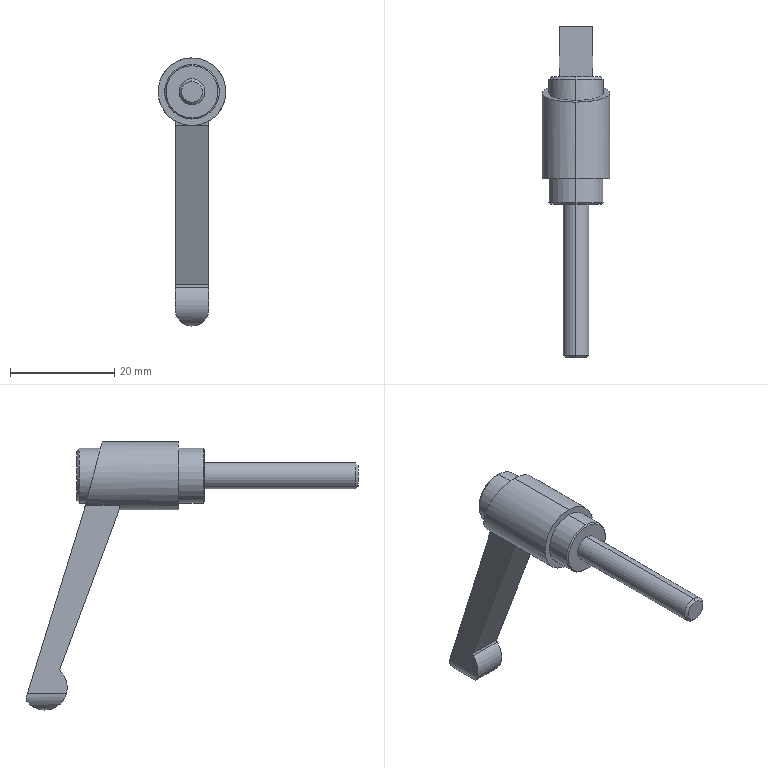Part | NX | features BREP 1 | 1 solid | 31 faces | box 13 x 63.763 x 51.5 mm | volume 4921 mm3 | cylinder 14 | plane 11 | cone 6 | commonest cylinder face diameters 10.5 x4 5 x2 6.5 x2 8.667 x2 13 x2 1 x1
STEP:
#1=CARTESIAN_POINT('',(0.,0.,5.));
#2=VERTEX_POINT('',#1);
#3=CARTESIAN_POINT('',(0.,0.,-5.));
#4=VERTEX_POINT('',#3);
#5=CARTESIAN_POINT('',(0.,0.,0.));
#6=DIRECTION('',(0.,-1.,0.));
#7=DIRECTION('',(0.,0.,1.));
#8=AXIS2_PLACEMENT_3D('',#5,#6,#7);
#9=CIRCLE('',#8,5.);
#10=EDGE_CURVE('',#2,#4,#9,.T.);
#11=ORIENTED_EDGE('',*,*,#10,.T.);
#12=CARTESIAN_POINT('',(0.,0.,0.));
#13=DIRECTION('',(0.,-1.,0.));
#14=DIRECTION('',(0.,0.,-1.));
#15=AXIS2_PLACEMENT_3D('',#12,#13,#14);
#16=CIRCLE('',#15,5.);
#17=EDGE_CURVE('',#4,#2,#16,.T.);
#18=ORIENTED_EDGE('',*,*,#17,.T.);
#19=EDGE_LOOP('',(#11,#18));
#20=FACE_BOUND('',#19,.T.);
#21=CARTESIAN_POINT('',(0.,0.,2.5));
#22=VERTEX_POINT('',#21);
#23=CARTESIAN_POINT('',(0.,0.,-2.5));
#24=VERTEX_POINT('',#23);
#25=CARTESIAN_POINT('',(0.,0.,0.));
#26=DIRECTION('',(0.,1.,0.));
#27=DIRECTION('',(0.,0.,1.));
#28=AXIS2_PLACEMENT_3D('',#25,#26,#27);
#29=CIRCLE('',#28,2.5);
#30=EDGE_CURVE('',#22,#24,#29,.T.);
#31=ORIENTED_EDGE('',*,*,#30,.T.);
#32=CARTESIAN_POINT('',(0.,0.,0.));
#33=DIRECTION('',(0.,1.,0.));
#34=DIRECTION('',(0.,0.,-1.));
#35=AXIS2_PLACEMENT_3D('',#32,#33,#34);
#36=CIRCLE('',#35,2.5);
#37=EDGE_CURVE('',#24,#22,#36,.T.);
#38=ORIENTED_EDGE('',*,*,#37,.T.);
#39=EDGE_LOOP('',(#31,#38));
#40=FACE_BOUND('',#39,.T.);
#41=CARTESIAN_POINT('',(0.,0.,-5.));
#42=DIRECTION('',(0.,1.,0.));
#43=DIRECTION('',(1.,0.,0.));
#44=AXIS2_PLACEMENT_3D('',#41,#42,#43);
#45=PLANE('',#44);
#46=ADVANCED_FACE('',(#20,#40),#45,.F.);
#47=CARTESIAN_POINT('',(0.,0.25,5.25));
#48=VERTEX_POINT('',#47);
#49=CARTESIAN_POINT('',(0.,0.,5.));
#50=DIRECTION('',(0.,0.7071,0.7071));
#51=VECTOR('',#50,1000.);
#52=LINE('',#49,#51);
#53=EDGE_CURVE('',#48,#2,#52,.F.);
#54=ORIENTED_EDGE('',*,*,#53,.T.);
#55=ORIENTED_EDGE('',*,*,#17,.F.);
#56=CARTESIAN_POINT('',(0.,0.25,-5.25));
#57=VERTEX_POINT('',#56);
#58=CARTESIAN_POINT('',(0.,0.,-5.));
#59=DIRECTION('',(0.,0.7071,-0.7071));
#60=VECTOR('',#59,1000.);
#61=LINE('',#58,#60);
#62=EDGE_CURVE('',#57,#4,#61,.F.);
#63=ORIENTED_EDGE('',*,*,#62,.F.);
#64=CARTESIAN_POINT('',(0.,0.25,0.));
#65=DIRECTION('',(0.,-1.,0.));
#66=DIRECTION('',(0.,0.,-1.));
#67=AXIS2_PLACEMENT_3D('',#64,#65,#66);
#68=CIRCLE('',#67,5.25);
#69=EDGE_CURVE('',#57,#48,#68,.T.);
#70=ORIENTED_EDGE('',*,*,#69,.T.);
#71=EDGE_LOOP('',(#54,#55,#63,#70));
#72=FACE_BOUND('',#71,.T.);
#73=CARTESIAN_POINT('',(0.,0.125,0.));
#74=DIRECTION('',(0.,1.,0.));
#75=DIRECTION('',(0.,0.,1.));
#76=AXIS2_PLACEMENT_3D('',#73,#74,#75);
#77=CONICAL_SURFACE('',#76,5.125,0.7854);
#78=ADVANCED_FACE('',(#72),#77,.T.);
#79=CARTESIAN_POINT('',(0.,4.9,5.25));
#80=VERTEX_POINT('',#79);
#81=CARTESIAN_POINT('',(0.,0.25,5.25));
#82=DIRECTION('',(0.,1.,0.));
#83=VECTOR('',#82,1000.);
#84=LINE('',#81,#83);
#85=EDGE_CURVE('',#80,#48,#84,.F.);
#86=ORIENTED_EDGE('',*,*,#85,.T.);
#87=ORIENTED_EDGE('',*,*,#69,.F.);
#88=CARTESIAN_POINT('',(0.,4.9,-5.25));
#89=VERTEX_POINT('',#88);
#90=CARTESIAN_POINT('',(0.,0.25,-5.25));
#91=DIRECTION('',(0.,1.,0.));
#92=VECTOR('',#91,1000.);
#93=LINE('',#90,#92);
#94=EDGE_CURVE('',#89,#57,#93,.F.);
#95=ORIENTED_EDGE('',*,*,#94,.F.);
#96=CARTESIAN_POINT('',(0.,4.9,0.));
#97=DIRECTION('',(0.,1.,0.));
#98=DIRECTION('',(0.,0.,1.));
#99=AXIS2_PLACEMENT_3D('',#96,#97,#98);
#100=CIRCLE('',#99,5.25);
#101=EDGE_CURVE('',#80,#89,#100,.T.);
#102=ORIENTED_EDGE('',*,*,#101,.F.);
#103=EDGE_LOOP('',(#86,#87,#95,#102));
#104=FACE_BOUND('',#103,.T.);
#105=CARTESIAN_POINT('',(0.,-29.5,0.));
#106=DIRECTION('',(0.,1.,0.));
#107=DIRECTION('',(0.,0.,-1.));
#108=AXIS2_PLACEMENT_3D('',#105,#106,#107);
#109=CYLINDRICAL_SURFACE('',#108,5.25);
#110=ADVANCED_FACE('',(#104),#109,.T.);
#111=CARTESIAN_POINT('',(0.,4.9,6.5));
#112=VERTEX_POINT('',#111);
#113=CARTESIAN_POINT('',(0.,4.9,-6.5));
#114=VERTEX_POINT('',#113);
#115=CARTESIAN_POINT('',(0.,4.9,0.));
#116=DIRECTION('',(0.,-1.,0.));
#117=DIRECTION('',(0.,0.,1.));
#118=AXIS2_PLACEMENT_3D('',#115,#116,#117);
#119=CIRCLE('',#118,6.5);
#120=EDGE_CURVE('',#112,#114,#119,.T.);
#121=ORIENTED_EDGE('',*,*,#120,.T.);
#122=CARTESIAN_POINT('',(0.,4.9,0.));
#123=DIRECTION('',(0.,-1.,0.));
#124=DIRECTION('',(0.,0.,-1.));
#125=AXIS2_PLACEMENT_3D('',#122,#123,#124);
#126=CIRCLE('',#125,6.5);
#127=EDGE_CURVE('',#114,#112,#126,.T.);
#128=ORIENTED_EDGE('',*,*,#127,.T.);
#129=EDGE_LOOP('',(#121,#128));
#130=FACE_BOUND('',#129,.T.);
#131=ORIENTED_EDGE('',*,*,#101,.T.);
#132=CARTESIAN_POINT('',(0.,4.9,0.));
#133=DIRECTION('',(0.,1.,0.));
#134=DIRECTION('',(0.,0.,-1.));
#135=AXIS2_PLACEMENT_3D('',#132,#133,#134);
#136=CIRCLE('',#135,5.25);
#137=EDGE_CURVE('',#89,#80,#136,.T.);
#138=ORIENTED_EDGE('',*,*,#137,.T.);
#139=EDGE_LOOP('',(#131,#138));
#140=FACE_BOUND('',#139,.T.);
#141=CARTESIAN_POINT('',(0.,4.9,-6.5));
#142=DIRECTION('',(0.,1.,0.));
#143=DIRECTION('',(1.,0.,0.));
#144=AXIS2_PLACEMENT_3D('',#141,#142,#143);
#145=PLANE('',#144);
#146=ADVANCED_FACE('',(#130,#140),#145,.F.);
#147=CARTESIAN_POINT('',(0.,19.6,6.5));
#148=VERTEX_POINT('',#147);
#149=CARTESIAN_POINT('',(0.,4.9,6.5));
#150=DIRECTION('',(0.,1.,0.));
#151=VECTOR('',#150,1000.);
#152=LINE('',#149,#151);
#153=EDGE_CURVE('',#148,#112,#152,.F.);
#154=ORIENTED_EDGE('',*,*,#153,.T.);
#155=ORIENTED_EDGE('',*,*,#127,.F.);
#156=CARTESIAN_POINT('',(0.,16.333,-6.5));
#157=VERTEX_POINT('',#156);
#158=CARTESIAN_POINT('',(0.,4.9,-6.5));
#159=DIRECTION('',(0.,1.,0.));
#160=VECTOR('',#159,1000.);
#161=LINE('',#158,#160);
#162=EDGE_CURVE('',#157,#114,#161,.F.);
#163=ORIENTED_EDGE('',*,*,#162,.F.);
#164=CARTESIAN_POINT('',(3.25,16.333,-5.629));
#165=VERTEX_POINT('',#164);
#166=CARTESIAN_POINT('',(0.,16.333,0.));
#167=DIRECTION('',(0.,1.,0.));
#168=DIRECTION('',(0.5,0.,-0.866));
#169=AXIS2_PLACEMENT_3D('',#166,#167,#168);
#170=CIRCLE('',#169,6.5);
#171=EDGE_CURVE('',#165,#157,#170,.T.);
#172=ORIENTED_EDGE('',*,*,#171,.F.);
#173=CARTESIAN_POINT('',(3.25,22.814,-5.629));
#174=VERTEX_POINT('',#173);
#175=CARTESIAN_POINT('',(3.25,16.333,-5.629));
#176=DIRECTION('',(0.,1.,0.));
#177=VECTOR('',#176,1000.);
#178=LINE('',#175,#177);
#179=EDGE_CURVE('',#165,#174,#178,.T.);
#180=ORIENTED_EDGE('',*,*,#179,.T.);
#181=CARTESIAN_POINT('',(0.,23.083,-6.5));
#182=VERTEX_POINT('',#181);
#183=CARTESIAN_POINT('',(0.,23.083,-6.5));
#184=CARTESIAN_POINT('',(1.126,23.083,-6.5));
#185=CARTESIAN_POINT('',(2.25,22.992,-6.206));
#186=CARTESIAN_POINT('',(3.25,22.814,-5.629));
#187=B_SPLINE_CURVE_WITH_KNOTS('',3,(#183,#184,#185,#186),.UNSPECIFIED.,.F.,.F.,(4,4),(0.,1.),.UNSPECIFIED.);
#188=EDGE_CURVE('',#174,#182,#187,.F.);
#189=ORIENTED_EDGE('',*,*,#188,.T.);
#190=CARTESIAN_POINT('',(0.,19.6,6.5));
#191=CARTESIAN_POINT('',(0.8361,19.6,6.5));
#192=CARTESIAN_POINT('',(2.441,19.681,6.199));
#193=CARTESIAN_POINT('',(4.728,20.071,4.744));
#194=CARTESIAN_POINT('',(6.224,20.698,2.403));
#195=CARTESIAN_POINT('',(6.638,21.342,0.00000182));
#196=CARTESIAN_POINT('',(6.224,21.986,-2.403));
#197=CARTESIAN_POINT('',(4.728,22.613,-4.744));
#198=CARTESIAN_POINT('',(2.441,23.003,-6.199));
#199=CARTESIAN_POINT('',(0.8365,23.083,-6.5));
#200=CARTESIAN_POINT('',(0.,23.083,-6.5));
#201=B_SPLINE_CURVE_WITH_KNOTS('',3,(#190,#191,#192,#193,#194,#195,#196,#197,#198,#199,#200),.UNSPECIFIED.,.F.,.F.,(4,1,1,1,1,1,1,1,4),(0.,0.125,0.25,0.375,0.5,0.625,0.75,0.875,1.),.UNSPECIFIED.);
#202=EDGE_CURVE('',#182,#148,#201,.F.);
#203=ORIENTED_EDGE('',*,*,#202,.T.);
#204=EDGE_LOOP('',(#154,#155,#163,#172,#180,#189,#203));
#205=FACE_BOUND('',#204,.T.);
#206=CARTESIAN_POINT('',(0.,-29.5,0.));
#207=DIRECTION('',(0.,1.,0.));
#208=DIRECTION('',(0.,0.,-1.));
#209=AXIS2_PLACEMENT_3D('',#206,#207,#208);
#210=CYLINDRICAL_SURFACE('',#209,6.5);
#211=ADVANCED_FACE('',(#205),#210,.T.);
#212=ORIENTED_EDGE('',*,*,#202,.F.);
#213=CARTESIAN_POINT('',(0.,23.083,-6.5));
#214=CARTESIAN_POINT('',(-0.8361,23.083,-6.5));
#215=CARTESIAN_POINT('',(-2.441,23.003,-6.199));
#216=CARTESIAN_POINT('',(-4.728,22.613,-4.744));
#217=CARTESIAN_POINT('',(-6.224,21.986,-2.403));
#218=CARTESIAN_POINT('',(-6.638,21.342,-0.00000182));
#219=CARTESIAN_POINT('',(-6.224,20.698,2.403));
#220=CARTESIAN_POINT('',(-4.728,20.071,4.744));
#221=CARTESIAN_POINT('',(-2.441,19.681,6.199));
#222=CARTESIAN_POINT('',(-0.8365,19.6,6.5));
#223=CARTESIAN_POINT('',(0.,19.6,6.5));
#224=B_SPLINE_CURVE_WITH_KNOTS('',3,(#213,#214,#215,#216,#217,#218,#219,#220,#221,#222,#223),.UNSPECIFIED.,.F.,.F.,(4,1,1,1,1,1,1,1,4),(0.,0.125,0.25,0.375,0.5,0.625,0.75,0.875,1.),.UNSPECIFIED.);
#225=EDGE_CURVE('',#148,#182,#224,.F.);
#226=ORIENTED_EDGE('',*,*,#225,.F.);
#227=EDGE_LOOP('',(#212,#226));
#228=FACE_BOUND('',#227,.T.);
#229=CARTESIAN_POINT('',(0.,19.935,5.25));
#230=VERTEX_POINT('',#229);
#231=CARTESIAN_POINT('',(0.,22.748,-5.25));
#232=VERTEX_POINT('',#231);
#233=CARTESIAN_POINT('',(0.,22.748,-5.25));
#234=CARTESIAN_POINT('',(0.6753,22.748,-5.25));
#235=CARTESIAN_POINT('',(1.972,22.683,-5.007));
#236=CARTESIAN_POINT('',(3.819,22.368,-3.832));
#237=CARTESIAN_POINT('',(5.027,21.862,-1.941));
#238=CARTESIAN_POINT('',(5.361,21.342,-0.00000147));
#239=CARTESIAN_POINT('',(5.027,20.822,1.941));
#240=CARTESIAN_POINT('',(3.819,20.315,3.832));
#241=CARTESIAN_POINT('',(1.972,20.,5.007));
#242=CARTESIAN_POINT('',(0.6757,19.935,5.25));
#243=CARTESIAN_POINT('',(0.,19.935,5.25));
#244=B_SPLINE_CURVE_WITH_KNOTS('',3,(#233,#234,#235,#236,#237,#238,#239,#240,#241,#242,#243),.UNSPECIFIED.,.F.,.F.,(4,1,1,1,1,1,1,1,4),(0.,0.125,0.25,0.375,0.5,0.625,0.75,0.875,1.),.UNSPECIFIED.);
#245=EDGE_CURVE('',#230,#232,#244,.F.);
#246=ORIENTED_EDGE('',*,*,#245,.F.);
#247=CARTESIAN_POINT('',(0.,19.935,5.25));
#248=CARTESIAN_POINT('',(-0.6753,19.935,5.25));
#249=CARTESIAN_POINT('',(-1.972,20.,5.007));
#250=CARTESIAN_POINT('',(-3.819,20.315,3.832));
#251=CARTESIAN_POINT('',(-5.027,20.822,1.941));
#252=CARTESIAN_POINT('',(-5.361,21.342,0.00000147));
#253=CARTESIAN_POINT('',(-5.027,21.862,-1.941));
#254=CARTESIAN_POINT('',(-3.819,22.368,-3.832));
#255=CARTESIAN_POINT('',(-1.972,22.683,-5.007));
#256=CARTESIAN_POINT('',(-0.6757,22.748,-5.25));
#257=CARTESIAN_POINT('',(0.,22.748,-5.25));
#258=B_SPLINE_CURVE_WITH_KNOTS('',3,(#247,#248,#249,#250,#251,#252,#253,#254,#255,#256,#257),.UNSPECIFIED.,.F.,.F.,(4,1,1,1,1,1,1,1,4),(0.,0.125,0.25,0.375,0.5,0.625,0.75,0.875,1.),.UNSPECIFIED.);
#259=EDGE_CURVE('',#232,#230,#258,.F.);
#260=ORIENTED_EDGE('',*,*,#259,.F.);
#261=EDGE_LOOP('',(#246,#260));
#262=FACE_BOUND('',#261,.T.);
#263=CARTESIAN_POINT('',(13.,19.6,6.5));
#264=DIRECTION('',(0.,0.9659,0.2588));
#265=DIRECTION('',(1.,0.,0.));
#266=AXIS2_PLACEMENT_3D('',#263,#264,#265);
#267=PLANE('',#266);
#268=ADVANCED_FACE('',(#228,#262),#267,.T.);
#269=CARTESIAN_POINT('',(-3.25,22.814,-5.629));
#270=VERTEX_POINT('',#269);
#271=CARTESIAN_POINT('',(-3.25,22.814,-5.629));
#272=CARTESIAN_POINT('',(-2.251,22.992,-6.206));
#273=CARTESIAN_POINT('',(-1.127,23.083,-6.5));
#274=CARTESIAN_POINT('',(0.,23.083,-6.5));
#275=B_SPLINE_CURVE_WITH_KNOTS('',3,(#271,#272,#273,#274),.UNSPECIFIED.,.F.,.F.,(4,4),(0.,1.),.UNSPECIFIED.);
#276=EDGE_CURVE('',#182,#270,#275,.F.);
#277=ORIENTED_EDGE('',*,*,#276,.T.);
#278=CARTESIAN_POINT('',(-3.25,16.333,-5.629));
#279=VERTEX_POINT('',#278);
#280=CARTESIAN_POINT('',(-3.25,22.814,-5.629));
#281=DIRECTION('',(0.,-1.,0.));
#282=VECTOR('',#281,1000.);
#283=LINE('',#280,#282);
#284=EDGE_CURVE('',#270,#279,#283,.T.);
#285=ORIENTED_EDGE('',*,*,#284,.T.);
#286=CARTESIAN_POINT('',(0.,16.333,0.));
#287=DIRECTION('',(0.,1.,0.));
#288=DIRECTION('',(0.,0.,-1.));
#289=AXIS2_PLACEMENT_3D('',#286,#287,#288);
#290=CIRCLE('',#289,6.5);
#291=EDGE_CURVE('',#157,#279,#290,.T.);
#292=ORIENTED_EDGE('',*,*,#291,.F.);
#293=ORIENTED_EDGE('',*,*,#162,.T.);
#294=ORIENTED_EDGE('',*,*,#120,.F.);
#295=ORIENTED_EDGE('',*,*,#153,.F.);
#296=ORIENTED_EDGE('',*,*,#225,.T.);
#297=EDGE_LOOP('',(#277,#285,#292,#293,#294,#295,#296));
#298=FACE_BOUND('',#297,.T.);
#299=CARTESIAN_POINT('',(0.,-29.5,0.));
#300=DIRECTION('',(0.,1.,0.));
#301=DIRECTION('',(0.,0.,-1.));
#302=AXIS2_PLACEMENT_3D('',#299,#300,#301);
#303=CYLINDRICAL_SURFACE('',#302,6.5);
#304=ADVANCED_FACE('',(#298),#303,.T.);
#305=ORIENTED_EDGE('',*,*,#291,.T.);
#306=CARTESIAN_POINT('',(-3.25,16.333,-6.5));
#307=VERTEX_POINT('',#306);
#308=CARTESIAN_POINT('',(-3.25,16.333,-6.5));
#309=DIRECTION('',(0.,0.,1.));
#310=VECTOR('',#309,1000.);
#311=LINE('',#308,#310);
#312=EDGE_CURVE('',#307,#279,#311,.T.);
#313=ORIENTED_EDGE('',*,*,#312,.F.);
#314=CARTESIAN_POINT('',(-3.25,16.333,-6.5));
#315=DIRECTION('',(1.,0.,0.));
#316=VECTOR('',#315,1000.);
#317=LINE('',#314,#316);
#318=EDGE_CURVE('',#307,#157,#317,.T.);
#319=ORIENTED_EDGE('',*,*,#318,.T.);
#320=EDGE_LOOP('',(#305,#313,#319));
#321=FACE_BOUND('',#320,.T.);
#322=CARTESIAN_POINT('',(3.25,16.333,0.));
#323=DIRECTION('',(0.,1.,0.));
#324=DIRECTION('',(1.,0.,0.));
#325=AXIS2_PLACEMENT_3D('',#322,#323,#324);
#326=PLANE('',#325);
#327=ADVANCED_FACE('',(#321),#326,.F.);
#328=CARTESIAN_POINT('',(3.25,27.716,-37.076));
#329=VERTEX_POINT('',#328);
#330=CARTESIAN_POINT('',(-3.25,27.716,-37.076));
#331=VERTEX_POINT('',#330);
#332=CARTESIAN_POINT('',(3.25,27.716,-37.076));
#333=DIRECTION('',(-1.,0.,0.));
#334=VECTOR('',#333,1000.);
#335=LINE('',#332,#334);
#336=EDGE_CURVE('',#329,#331,#335,.T.);
#337=ORIENTED_EDGE('',*,*,#336,.F.);
#338=CARTESIAN_POINT('',(3.25,16.333,-6.5));
#339=VERTEX_POINT('',#338);
#340=CARTESIAN_POINT('',(3.25,16.333,-6.5));
#341=DIRECTION('',(0.,0.3489,-0.9372));
#342=VECTOR('',#341,1000.);
#343=LINE('',#340,#342);
#344=EDGE_CURVE('',#339,#329,#343,.T.);
#345=ORIENTED_EDGE('',*,*,#344,.F.);
#346=CARTESIAN_POINT('',(0.,16.333,-6.5));
#347=DIRECTION('',(1.,0.,0.));
#348=VECTOR('',#347,1000.);
#349=LINE('',#346,#348);
#350=EDGE_CURVE('',#157,#339,#349,.T.);
#351=ORIENTED_EDGE('',*,*,#350,.F.);
#352=ORIENTED_EDGE('',*,*,#318,.F.);
#353=CARTESIAN_POINT('',(-3.25,27.716,-37.076));
#354=DIRECTION('',(0.,-0.3489,0.9372));
#355=VECTOR('',#354,1000.);
#356=LINE('',#353,#355);
#357=EDGE_CURVE('',#331,#307,#356,.T.);
#358=ORIENTED_EDGE('',*,*,#357,.F.);
#359=EDGE_LOOP('',(#337,#345,#351,#352,#358));
#360=FACE_BOUND('',#359,.T.);
#361=CARTESIAN_POINT('',(3.25,16.333,-6.5));
#362=DIRECTION('',(0.,0.9372,0.3489));
#363=DIRECTION('',(1.,0.,0.));
#364=AXIS2_PLACEMENT_3D('',#361,#362,#363);
#365=PLANE('',#364);
#366=ADVANCED_FACE('',(#360),#365,.F.);
#367=CARTESIAN_POINT('',(-3.25,26.471,-41.75));
#368=VERTEX_POINT('',#367);
#369=CARTESIAN_POINT('',(-3.25,27.602,-37.604));
#370=VERTEX_POINT('',#369);
#371=CARTESIAN_POINT('',(-3.25,30.667,-40.667));
#372=DIRECTION('',(-1.,0.,0.));
#373=DIRECTION('',(0.,-0.9682,-0.25));
#374=AXIS2_PLACEMENT_3D('',#371,#372,#373);
#375=CIRCLE('',#374,4.333);
#376=EDGE_CURVE('',#368,#370,#375,.T.);
#377=ORIENTED_EDGE('',*,*,#376,.T.);
#378=CARTESIAN_POINT('',(-3.25,27.248,-37.25));
#379=DIRECTION('',(1.,0.,0.));
#380=DIRECTION('',(0.,0.7073,-0.7069));
#381=AXIS2_PLACEMENT_3D('',#378,#379,#380);
#382=CIRCLE('',#381,0.5);
#383=EDGE_CURVE('',#370,#331,#382,.T.);
#384=ORIENTED_EDGE('',*,*,#383,.T.);
#385=ORIENTED_EDGE('',*,*,#357,.T.);
#386=ORIENTED_EDGE('',*,*,#312,.T.);
#387=ORIENTED_EDGE('',*,*,#284,.F.);
#388=CARTESIAN_POINT('',(-3.25,33.994,-41.75));
#389=VERTEX_POINT('',#388);
#390=CARTESIAN_POINT('',(-3.25,22.814,-5.629));
#391=DIRECTION('',(0.,0.2957,-0.9553));
#392=VECTOR('',#391,1000.);
#393=LINE('',#390,#392);
#394=EDGE_CURVE('',#270,#389,#393,.T.);
#395=ORIENTED_EDGE('',*,*,#394,.T.);
#396=CARTESIAN_POINT('',(-3.25,26.471,-41.75));
#397=DIRECTION('',(0.,1.,0.));
#398=VECTOR('',#397,1000.);
#399=LINE('',#396,#398);
#400=EDGE_CURVE('',#368,#389,#399,.T.);
#401=ORIENTED_EDGE('',*,*,#400,.F.);
#402=EDGE_LOOP('',(#377,#384,#385,#386,#387,#395,#401));
#403=FACE_BOUND('',#402,.T.);
#404=CARTESIAN_POINT('',(-3.25,27.248,-37.25));
#405=DIRECTION('',(1.,0.,0.));
#406=DIRECTION('',(0.,1.,0.));
#407=AXIS2_PLACEMENT_3D('',#404,#405,#406);
#408=PLANE('',#407);
#409=ADVANCED_FACE('',(#403),#408,.F.);
#410=CARTESIAN_POINT('',(-2.806,34.038,-43.389));
#411=VERTEX_POINT('',#410);
#412=CARTESIAN_POINT('',(0.,30.667,-45.));
#413=VERTEX_POINT('',#412);
#414=CARTESIAN_POINT('',(-2.806,34.038,-43.389));
#415=CARTESIAN_POINT('',(-2.678,33.861,-43.609));
#416=CARTESIAN_POINT('',(-2.372,33.462,-44.023));
#417=CARTESIAN_POINT('',(-1.814,32.783,-44.467));
#418=CARTESIAN_POINT('',(-1.358,32.243,-44.715));
#419=CARTESIAN_POINT('',(-0.888,31.694,-44.885));
#420=CARTESIAN_POINT('',(-0.5786,31.334,-44.956));
#421=CARTESIAN_POINT('',(-0.2049,30.903,-45.));
#422=CARTESIAN_POINT('',(0.,30.667,-45.));
#423=B_SPLINE_CURVE_WITH_KNOTS('',3,(#414,#415,#416,#417,#418,#419,#420,#421,#422),.UNSPECIFIED.,.F.,.F.,(4,1,1,1,1,1,4),(0.,0.25,0.5,0.625,0.75,0.875,1.),.UNSPECIFIED.);
#424=EDGE_CURVE('',#411,#413,#423,.T.);
#425=ORIENTED_EDGE('',*,*,#424,.T.);
#426=CARTESIAN_POINT('',(0.,30.667,-45.));
#427=CARTESIAN_POINT('',(-0.1682,30.472,-45.));
#428=CARTESIAN_POINT('',(-0.4752,30.118,-44.97));
#429=CARTESIAN_POINT('',(-0.7263,29.827,-44.924));
#430=CARTESIAN_POINT('',(-1.124,29.365,-44.807));
#431=CARTESIAN_POINT('',(-1.501,28.922,-44.646));
#432=CARTESIAN_POINT('',(-2.021,28.302,-44.325));
#433=CARTESIAN_POINT('',(-2.602,27.582,-43.769));
#434=CARTESIAN_POINT('',(-3.141,26.84,-42.835));
#435=CARTESIAN_POINT('',(-3.25,26.567,-42.123));
#436=CARTESIAN_POINT('',(-3.25,26.471,-41.75));
#437=B_SPLINE_CURVE_WITH_KNOTS('',3,(#426,#427,#428,#429,#430,#431,#432,#433,#434,#435,#436),.UNSPECIFIED.,.F.,.F.,(4,1,1,1,1,1,1,1,4),(0.,0.0625,0.125,0.1875,0.25,0.375,0.5,0.75,1.),.UNSPECIFIED.);
#438=EDGE_CURVE('',#413,#368,#437,.T.);
#439=ORIENTED_EDGE('',*,*,#438,.T.);
#440=ORIENTED_EDGE('',*,*,#400,.T.);
#441=CARTESIAN_POINT('',(-3.17,34.215,-42.465));
#442=VERTEX_POINT('',#441);
#443=CARTESIAN_POINT('',(-3.17,34.215,-42.465));
#444=CARTESIAN_POINT('',(-3.223,34.143,-42.23));
#445=CARTESIAN_POINT('',(-3.25,34.069,-41.991));
#446=CARTESIAN_POINT('',(-3.25,33.994,-41.75));
#447=B_SPLINE_CURVE_WITH_KNOTS('',3,(#443,#444,#445,#446),.UNSPECIFIED.,.F.,.F.,(4,4),(0.,1.),.UNSPECIFIED.);
#448=EDGE_CURVE('',#389,#442,#447,.F.);
#449=ORIENTED_EDGE('',*,*,#448,.T.);
#450=CARTESIAN_POINT('',(-3.17,34.215,-42.465));
#451=CARTESIAN_POINT('',(-3.1,34.312,-42.778));
#452=CARTESIAN_POINT('',(-2.96,34.25,-43.126));
#453=CARTESIAN_POINT('',(-2.806,34.038,-43.389));
#454=B_SPLINE_CURVE_WITH_KNOTS('',3,(#450,#451,#452,#453),.UNSPECIFIED.,.F.,.F.,(4,4),(0.,1.),.UNSPECIFIED.);
#455=EDGE_CURVE('',#442,#411,#454,.T.);
#456=ORIENTED_EDGE('',*,*,#455,.T.);
#457=EDGE_LOOP('',(#425,#439,#440,#449,#456));
#458=FACE_BOUND('',#457,.T.);
#459=CARTESIAN_POINT('',(0.,35.,-41.75));
#460=DIRECTION('',(0.,1.,0.));
#461=DIRECTION('',(0.,0.,-1.));
#462=AXIS2_PLACEMENT_3D('',#459,#460,#461);
#463=CYLINDRICAL_SURFACE('',#462,3.25);
#464=ADVANCED_FACE('',(#458),#463,.T.);
#465=ORIENTED_EDGE('',*,*,#455,.F.);
#466=CARTESIAN_POINT('',(3.17,34.215,-42.465));
#467=VERTEX_POINT('',#466);
#468=CARTESIAN_POINT('',(-3.17,34.215,-42.465));
#469=DIRECTION('',(1.,0.,0.));
#470=VECTOR('',#469,1000.);
#471=LINE('',#468,#470);
#472=EDGE_CURVE('',#442,#467,#471,.T.);
#473=ORIENTED_EDGE('',*,*,#472,.T.);
#474=CARTESIAN_POINT('',(2.806,34.038,-43.389));
#475=VERTEX_POINT('',#474);
#476=CARTESIAN_POINT('',(3.17,34.215,-42.465));
#477=CARTESIAN_POINT('',(3.137,34.261,-42.614));
#478=CARTESIAN_POINT('',(3.07,34.29,-42.851));
#479=CARTESIAN_POINT('',(2.909,34.161,-43.201));
#480=CARTESIAN_POINT('',(2.876,34.134,-43.27));
#481=CARTESIAN_POINT('',(2.806,34.038,-43.389));
#482=B_SPLINE_CURVE_WITH_KNOTS('',3,(#476,#477,#478,#479,#480,#481),.UNSPECIFIED.,.F.,.F.,(4,1,1,4),(0.,0.5,0.75,1.),.UNSPECIFIED.);
#483=EDGE_CURVE('',#467,#475,#482,.T.);
#484=ORIENTED_EDGE('',*,*,#483,.T.);
#485=CARTESIAN_POINT('',(-2.806,34.038,-43.389));
#486=DIRECTION('',(1.,0.,0.));
#487=VECTOR('',#486,1000.);
#488=LINE('',#485,#487);
#489=EDGE_CURVE('',#411,#475,#488,.T.);
#490=ORIENTED_EDGE('',*,*,#489,.F.);
#491=EDGE_LOOP('',(#465,#473,#484,#490));
#492=FACE_BOUND('',#491,.T.);
#493=CARTESIAN_POINT('',(3.25,33.26,-42.761));
#494=DIRECTION('',(1.,0.,0.));
#495=DIRECTION('',(0.,0.,1.));
#496=AXIS2_PLACEMENT_3D('',#493,#494,#495);
#497=CYLINDRICAL_SURFACE('',#496,1.);
#498=ADVANCED_FACE('',(#492),#497,.T.);
#499=CARTESIAN_POINT('',(2.806,34.038,-43.389));
#500=CARTESIAN_POINT('',(2.68,33.863,-43.606));
#501=CARTESIAN_POINT('',(2.372,33.46,-44.024));
#502=CARTESIAN_POINT('',(1.814,32.783,-44.468));
#503=CARTESIAN_POINT('',(1.358,32.244,-44.714));
#504=CARTESIAN_POINT('',(0.9,31.708,-44.884));
#505=CARTESIAN_POINT('',(0.5922,31.35,-44.948));
#506=CARTESIAN_POINT('',(0.364,31.087,-44.983));
#507=CARTESIAN_POINT('',(0.1339,30.821,-45.));
#508=CARTESIAN_POINT('',(0.,30.667,-45.));
#509=B_SPLINE_CURVE_WITH_KNOTS('',3,(#499,#500,#501,#502,#503,#504,#505,#506,#507,#508),.UNSPECIFIED.,.F.,.F.,(4,1,1,1,1,1,1,4),(0.,0.25,0.5,0.625,0.75,0.875,0.9375,1.),.UNSPECIFIED.);
#510=EDGE_CURVE('',#413,#475,#509,.F.);
#511=ORIENTED_EDGE('',*,*,#510,.F.);
#512=ORIENTED_EDGE('',*,*,#424,.F.);
#513=ORIENTED_EDGE('',*,*,#489,.T.);
#514=EDGE_LOOP('',(#511,#512,#513));
#515=FACE_BOUND('',#514,.T.);
#516=CARTESIAN_POINT('',(3.25,30.667,-40.667));
#517=DIRECTION('',(1.,0.,0.));
#518=DIRECTION('',(0.,0.,1.));
#519=AXIS2_PLACEMENT_3D('',#516,#517,#518);
#520=CYLINDRICAL_SURFACE('',#519,4.333);
#521=ADVANCED_FACE('',(#515),#520,.T.);
#522=ORIENTED_EDGE('',*,*,#483,.F.);
#523=CARTESIAN_POINT('',(3.25,33.994,-41.75));
#524=VERTEX_POINT('',#523);
#525=CARTESIAN_POINT('',(3.25,33.994,-41.75));
#526=CARTESIAN_POINT('',(3.25,34.069,-41.991));
#527=CARTESIAN_POINT('',(3.223,34.143,-42.23));
#528=CARTESIAN_POINT('',(3.17,34.215,-42.465));
#529=B_SPLINE_CURVE_WITH_KNOTS('',3,(#525,#526,#527,#528),.UNSPECIFIED.,.F.,.F.,(4,4),(0.,1.),.UNSPECIFIED.);
#530=EDGE_CURVE('',#467,#524,#529,.F.);
#531=ORIENTED_EDGE('',*,*,#530,.T.);
#532=CARTESIAN_POINT('',(3.25,26.471,-41.75));
#533=VERTEX_POINT('',#532);
#534=CARTESIAN_POINT('',(3.25,33.994,-41.75));
#535=DIRECTION('',(0.,-1.,0.));
#536=VECTOR('',#535,1000.);
#537=LINE('',#534,#536);
#538=EDGE_CURVE('',#524,#533,#537,.T.);
#539=ORIENTED_EDGE('',*,*,#538,.T.);
#540=CARTESIAN_POINT('',(3.25,26.471,-41.75));
#541=CARTESIAN_POINT('',(3.25,26.568,-42.126));
#542=CARTESIAN_POINT('',(3.136,26.848,-42.849));
#543=CARTESIAN_POINT('',(2.6,27.584,-43.77));
#544=CARTESIAN_POINT('',(2.021,28.302,-44.325));
#545=CARTESIAN_POINT('',(1.504,28.917,-44.644));
#546=CARTESIAN_POINT('',(1.127,29.361,-44.806));
#547=CARTESIAN_POINT('',(0.7302,29.822,-44.923));
#548=CARTESIAN_POINT('',(0.4774,30.116,-44.97));
#549=CARTESIAN_POINT('',(0.169,30.472,-45.));
#550=CARTESIAN_POINT('',(0.,30.667,-45.));
#551=B_SPLINE_CURVE_WITH_KNOTS('',3,(#540,#541,#542,#543,#544,#545,#546,#547,#548,#549,#550),.UNSPECIFIED.,.F.,.F.,(4,1,1,1,1,1,1,1,4),(0.,0.25,0.5,0.625,0.75,0.8125,0.875,0.9375,1.),.UNSPECIFIED.);
#552=EDGE_CURVE('',#533,#413,#551,.T.);
#553=ORIENTED_EDGE('',*,*,#552,.T.);
#554=ORIENTED_EDGE('',*,*,#510,.T.);
#555=EDGE_LOOP('',(#522,#531,#539,#553,#554));
#556=FACE_BOUND('',#555,.T.);
#557=CARTESIAN_POINT('',(0.,35.,-41.75));
#558=DIRECTION('',(0.,1.,0.));
#559=DIRECTION('',(0.,0.,-1.));
#560=AXIS2_PLACEMENT_3D('',#557,#558,#559);
#561=CYLINDRICAL_SURFACE('',#560,3.25);
#562=ADVANCED_FACE('',(#556),#561,.T.);
#563=ORIENTED_EDGE('',*,*,#438,.F.);
#564=ORIENTED_EDGE('',*,*,#552,.F.);
#565=CARTESIAN_POINT('',(3.25,27.602,-37.604));
#566=VERTEX_POINT('',#565);
#567=CARTESIAN_POINT('',(3.25,30.667,-40.667));
#568=DIRECTION('',(1.,0.,0.));
#569=DIRECTION('',(0.,-0.7073,0.7069));
#570=AXIS2_PLACEMENT_3D('',#567,#568,#569);
#571=CIRCLE('',#570,4.333);
#572=EDGE_CURVE('',#566,#533,#571,.T.);
#573=ORIENTED_EDGE('',*,*,#572,.F.);
#574=CARTESIAN_POINT('',(-3.25,27.602,-37.604));
#575=DIRECTION('',(1.,0.,0.));
#576=VECTOR('',#575,1000.);
#577=LINE('',#574,#576);
#578=EDGE_CURVE('',#370,#566,#577,.T.);
#579=ORIENTED_EDGE('',*,*,#578,.F.);
#580=ORIENTED_EDGE('',*,*,#376,.F.);
#581=EDGE_LOOP('',(#563,#564,#573,#579,#580));
#582=FACE_BOUND('',#581,.T.);
#583=CARTESIAN_POINT('',(3.25,30.667,-40.667));
#584=DIRECTION('',(1.,0.,0.));
#585=DIRECTION('',(0.,0.,1.));
#586=AXIS2_PLACEMENT_3D('',#583,#584,#585);
#587=CYLINDRICAL_SURFACE('',#586,4.333);
#588=ADVANCED_FACE('',(#582),#587,.T.);
#589=ORIENTED_EDGE('',*,*,#578,.T.);
#590=CARTESIAN_POINT('',(3.25,27.248,-37.25));
#591=DIRECTION('',(-1.,0.,0.));
#592=DIRECTION('',(0.,0.9372,0.3489));
#593=AXIS2_PLACEMENT_3D('',#590,#591,#592);
#594=CIRCLE('',#593,0.5);
#595=EDGE_CURVE('',#329,#566,#594,.T.);
#596=ORIENTED_EDGE('',*,*,#595,.F.);
#597=ORIENTED_EDGE('',*,*,#336,.T.);
#598=ORIENTED_EDGE('',*,*,#383,.F.);
#599=EDGE_LOOP('',(#589,#596,#597,#598));
#600=FACE_BOUND('',#599,.T.);
#601=CARTESIAN_POINT('',(3.25,27.248,-37.25));
#602=DIRECTION('',(1.,0.,0.));
#603=DIRECTION('',(0.,0.,1.));
#604=AXIS2_PLACEMENT_3D('',#601,#602,#603);
#605=CYLINDRICAL_SURFACE('',#604,0.5);
#606=ADVANCED_FACE('',(#600),#605,.F.);
#607=ORIENTED_EDGE('',*,*,#538,.F.);
#608=CARTESIAN_POINT('',(3.25,33.994,-41.75));
#609=DIRECTION('',(0.,-0.2957,0.9553));
#610=VECTOR('',#609,1000.);
#611=LINE('',#608,#610);
#612=EDGE_CURVE('',#524,#174,#611,.T.);
#613=ORIENTED_EDGE('',*,*,#612,.T.);
#614=ORIENTED_EDGE('',*,*,#179,.F.);
#615=CARTESIAN_POINT('',(3.25,16.333,-6.5));
#616=DIRECTION('',(0.,0.,1.));
#617=VECTOR('',#616,1000.);
#618=LINE('',#615,#617);
#619=EDGE_CURVE('',#339,#165,#618,.T.);
#620=ORIENTED_EDGE('',*,*,#619,.F.);
#621=ORIENTED_EDGE('',*,*,#344,.T.);
#622=ORIENTED_EDGE('',*,*,#595,.T.);
#623=ORIENTED_EDGE('',*,*,#572,.T.);
#624=EDGE_LOOP('',(#607,#613,#614,#620,#621,#622,#623));
#625=FACE_BOUND('',#624,.T.);
#626=CARTESIAN_POINT('',(3.25,27.248,-37.25));
#627=DIRECTION('',(1.,0.,0.));
#628=DIRECTION('',(0.,1.,0.));
#629=AXIS2_PLACEMENT_3D('',#626,#627,#628);
#630=PLANE('',#629);
#631=ADVANCED_FACE('',(#625),#630,.T.);
#632=ORIENTED_EDGE('',*,*,#171,.T.);
#633=ORIENTED_EDGE('',*,*,#350,.T.);
#634=ORIENTED_EDGE('',*,*,#619,.T.);
#635=EDGE_LOOP('',(#632,#633,#634));
#636=FACE_BOUND('',#635,.T.);
#637=CARTESIAN_POINT('',(3.25,16.333,0.));
#638=DIRECTION('',(0.,1.,0.));
#639=DIRECTION('',(1.,0.,0.));
#640=AXIS2_PLACEMENT_3D('',#637,#638,#639);
#641=PLANE('',#640);
#642=ADVANCED_FACE('',(#636),#641,.F.);
#643=ORIENTED_EDGE('',*,*,#530,.F.);
#644=ORIENTED_EDGE('',*,*,#472,.F.);
#645=ORIENTED_EDGE('',*,*,#448,.F.);
#646=ORIENTED_EDGE('',*,*,#394,.F.);
#647=ORIENTED_EDGE('',*,*,#276,.F.);
#648=ORIENTED_EDGE('',*,*,#188,.F.);
#649=ORIENTED_EDGE('',*,*,#612,.F.);
#650=EDGE_LOOP('',(#643,#644,#645,#646,#647,#648,#649));
#651=FACE_BOUND('',#650,.T.);
#652=CARTESIAN_POINT('',(3.25,34.215,-42.465));
#653=DIRECTION('',(0.,-0.9553,-0.2957));
#654=DIRECTION('',(0.,0.2957,-0.9553));
#655=AXIS2_PLACEMENT_3D('',#652,#653,#654);
#656=PLANE('',#655);
#657=ADVANCED_FACE('',(#651),#656,.F.);
#658=CARTESIAN_POINT('',(0.,24.,-5.25));
#659=VERTEX_POINT('',#658);
#660=CARTESIAN_POINT('',(0.,22.748,-5.25));
#661=DIRECTION('',(0.,1.,0.));
#662=VECTOR('',#661,1000.);
#663=LINE('',#660,#662);
#664=EDGE_CURVE('',#659,#232,#663,.F.);
#665=ORIENTED_EDGE('',*,*,#664,.T.);
#666=ORIENTED_EDGE('',*,*,#259,.T.);
#667=CARTESIAN_POINT('',(0.,24.,5.25));
#668=VERTEX_POINT('',#667);
#669=CARTESIAN_POINT('',(0.,19.935,5.25));
#670=DIRECTION('',(0.,1.,0.));
#671=VECTOR('',#670,1000.);
#672=LINE('',#669,#671);
#673=EDGE_CURVE('',#668,#230,#672,.F.);
#674=ORIENTED_EDGE('',*,*,#673,.F.);
#675=CARTESIAN_POINT('',(0.,24.,0.));
#676=DIRECTION('',(0.,1.,0.));
#677=DIRECTION('',(0.,0.,-1.));
#678=AXIS2_PLACEMENT_3D('',#675,#676,#677);
#679=CIRCLE('',#678,5.25);
#680=EDGE_CURVE('',#659,#668,#679,.T.);
#681=ORIENTED_EDGE('',*,*,#680,.F.);
#682=EDGE_LOOP('',(#665,#666,#674,#681));
#683=FACE_BOUND('',#682,.T.);
#684=CARTESIAN_POINT('',(0.,12.25,0.));
#685=DIRECTION('',(0.,1.,0.));
#686=DIRECTION('',(0.,0.,-1.));
#687=AXIS2_PLACEMENT_3D('',#684,#685,#686);
#688=CYLINDRICAL_SURFACE('',#687,5.25);
#689=ADVANCED_FACE('',(#683),#688,.T.);
#690=CARTESIAN_POINT('',(0.,24.5,4.75));
#691=VERTEX_POINT('',#690);
#692=CARTESIAN_POINT('',(0.,24.5,4.75));
#693=DIRECTION('',(0.,-0.7071,0.7071));
#694=VECTOR('',#693,1000.);
#695=LINE('',#692,#694);
#696=EDGE_CURVE('',#668,#691,#695,.F.);
#697=ORIENTED_EDGE('',*,*,#696,.T.);
#698=CARTESIAN_POINT('',(0.,24.5,-4.75));
#699=VERTEX_POINT('',#698);
#700=CARTESIAN_POINT('',(0.,24.5,0.));
#701=DIRECTION('',(0.,1.,0.));
#702=DIRECTION('',(0.,0.,-1.));
#703=AXIS2_PLACEMENT_3D('',#700,#701,#702);
#704=CIRCLE('',#703,4.75);
#705=EDGE_CURVE('',#699,#691,#704,.T.);
#706=ORIENTED_EDGE('',*,*,#705,.F.);
#707=CARTESIAN_POINT('',(0.,24.5,-4.75));
#708=DIRECTION('',(0.,-0.7071,-0.7071));
#709=VECTOR('',#708,1000.);
#710=LINE('',#707,#709);
#711=EDGE_CURVE('',#659,#699,#710,.F.);
#712=ORIENTED_EDGE('',*,*,#711,.F.);
#713=ORIENTED_EDGE('',*,*,#680,.T.);
#714=EDGE_LOOP('',(#697,#706,#712,#713));
#715=FACE_BOUND('',#714,.T.);
#716=CARTESIAN_POINT('',(0.,24.25,0.));
#717=DIRECTION('',(0.,-1.,0.));
#718=DIRECTION('',(0.,0.,-1.));
#719=AXIS2_PLACEMENT_3D('',#716,#717,#718);
#720=CONICAL_SURFACE('',#719,5.,0.7854);
#721=ADVANCED_FACE('',(#715),#720,.T.);
#722=ORIENTED_EDGE('',*,*,#711,.T.);
#723=CARTESIAN_POINT('',(0.,24.5,0.));
#724=DIRECTION('',(0.,1.,0.));
#725=DIRECTION('',(0.,0.,1.));
#726=AXIS2_PLACEMENT_3D('',#723,#724,#725);
#727=CIRCLE('',#726,4.75);
#728=EDGE_CURVE('',#691,#699,#727,.T.);
#729=ORIENTED_EDGE('',*,*,#728,.F.);
#730=ORIENTED_EDGE('',*,*,#696,.F.);
#731=CARTESIAN_POINT('',(0.,24.,0.));
#732=DIRECTION('',(0.,1.,0.));
#733=DIRECTION('',(0.,0.,1.));
#734=AXIS2_PLACEMENT_3D('',#731,#732,#733);
#735=CIRCLE('',#734,5.25);
#736=EDGE_CURVE('',#668,#659,#735,.T.);
#737=ORIENTED_EDGE('',*,*,#736,.T.);
#738=EDGE_LOOP('',(#722,#729,#730,#737));
#739=FACE_BOUND('',#738,.T.);
#740=CARTESIAN_POINT('',(0.,24.25,0.));
#741=DIRECTION('',(0.,-1.,0.));
#742=DIRECTION('',(0.,0.,-1.));
#743=AXIS2_PLACEMENT_3D('',#740,#741,#742);
#744=CONICAL_SURFACE('',#743,5.,0.7854);
#745=ADVANCED_FACE('',(#739),#744,.T.);
#746=ORIENTED_EDGE('',*,*,#673,.T.);
#747=ORIENTED_EDGE('',*,*,#245,.T.);
#748=ORIENTED_EDGE('',*,*,#664,.F.);
#749=ORIENTED_EDGE('',*,*,#736,.F.);
#750=EDGE_LOOP('',(#746,#747,#748,#749));
#751=FACE_BOUND('',#750,.T.);
#752=CARTESIAN_POINT('',(0.,12.25,0.));
#753=DIRECTION('',(0.,1.,0.));
#754=DIRECTION('',(0.,0.,-1.));
#755=AXIS2_PLACEMENT_3D('',#752,#753,#754);
#756=CYLINDRICAL_SURFACE('',#755,5.25);
#757=ADVANCED_FACE('',(#751),#756,.T.);
#758=ORIENTED_EDGE('',*,*,#728,.T.);
#759=ORIENTED_EDGE('',*,*,#705,.T.);
#760=EDGE_LOOP('',(#758,#759));
#761=FACE_BOUND('',#760,.T.);
#762=CARTESIAN_POINT('',(0.,24.5,0.));
#763=DIRECTION('',(0.,-1.,0.));
#764=DIRECTION('',(0.,0.,-1.));
#765=AXIS2_PLACEMENT_3D('',#762,#763,#764);
#766=PLANE('',#765);
#767=ADVANCED_FACE('',(#761),#766,.F.);
#768=ORIENTED_EDGE('',*,*,#94,.T.);
#769=CARTESIAN_POINT('',(0.,0.25,0.));
#770=DIRECTION('',(0.,-1.,0.));
#771=DIRECTION('',(0.,0.,1.));
#772=AXIS2_PLACEMENT_3D('',#769,#770,#771);
#773=CIRCLE('',#772,5.25);
#774=EDGE_CURVE('',#48,#57,#773,.T.);
#775=ORIENTED_EDGE('',*,*,#774,.F.);
#776=ORIENTED_EDGE('',*,*,#85,.F.);
#777=ORIENTED_EDGE('',*,*,#137,.F.);
#778=EDGE_LOOP('',(#768,#775,#776,#777));
#779=FACE_BOUND('',#778,.T.);
#780=CARTESIAN_POINT('',(0.,-29.5,0.));
#781=DIRECTION('',(0.,1.,0.));
#782=DIRECTION('',(0.,0.,-1.));
#783=AXIS2_PLACEMENT_3D('',#780,#781,#782);
#784=CYLINDRICAL_SURFACE('',#783,5.25);
#785=ADVANCED_FACE('',(#779),#784,.T.);
#786=ORIENTED_EDGE('',*,*,#62,.T.);
#787=ORIENTED_EDGE('',*,*,#10,.F.);
#788=ORIENTED_EDGE('',*,*,#53,.F.);
#789=ORIENTED_EDGE('',*,*,#774,.T.);
#790=EDGE_LOOP('',(#786,#787,#788,#789));
#791=FACE_BOUND('',#790,.T.);
#792=CARTESIAN_POINT('',(0.,0.125,0.));
#793=DIRECTION('',(0.,1.,0.));
#794=DIRECTION('',(0.,0.,1.));
#795=AXIS2_PLACEMENT_3D('',#792,#793,#794);
#796=CONICAL_SURFACE('',#795,5.125,0.7854);
#797=ADVANCED_FACE('',(#791),#796,.T.);
#798=CARTESIAN_POINT('',(0.,-29.009,-2.5));
#799=VERTEX_POINT('',#798);
#800=CARTESIAN_POINT('',(0.,-29.009,-2.5));
#801=DIRECTION('',(0.,1.,0.));
#802=VECTOR('',#801,1000.);
#803=LINE('',#800,#802);
#804=EDGE_CURVE('',#799,#24,#803,.T.);
#805=ORIENTED_EDGE('',*,*,#804,.F.);
#806=CARTESIAN_POINT('',(0.,-29.009,2.5));
#807=VERTEX_POINT('',#806);
#808=CARTESIAN_POINT('',(0.,-29.009,0.));
#809=DIRECTION('',(0.,-1.,0.));
#810=DIRECTION('',(0.,0.,1.));
#811=AXIS2_PLACEMENT_3D('',#808,#809,#810);
#812=CIRCLE('',#811,2.5);
#813=EDGE_CURVE('',#807,#799,#812,.T.);
#814=ORIENTED_EDGE('',*,*,#813,.F.);
#815=CARTESIAN_POINT('',(0.,-29.009,2.5));
#816=DIRECTION('',(0.,1.,0.));
#817=VECTOR('',#816,1000.);
#818=LINE('',#815,#817);
#819=EDGE_CURVE('',#807,#22,#818,.T.);
#820=ORIENTED_EDGE('',*,*,#819,.T.);
#821=ORIENTED_EDGE('',*,*,#37,.F.);
#822=EDGE_LOOP('',(#805,#814,#820,#821));
#823=FACE_BOUND('',#822,.T.);
#824=CARTESIAN_POINT('',(0.,-29.5,0.));
#825=DIRECTION('',(0.,1.,0.));
#826=DIRECTION('',(0.,0.,-1.));
#827=AXIS2_PLACEMENT_3D('',#824,#825,#826);
#828=CYLINDRICAL_SURFACE('',#827,2.5);
#829=ADVANCED_FACE('',(#823),#828,.T.);
#830=ORIENTED_EDGE('',*,*,#819,.F.);
#831=CARTESIAN_POINT('',(0.,-29.009,0.));
#832=DIRECTION('',(0.,-1.,0.));
#833=DIRECTION('',(0.,0.,-1.));
#834=AXIS2_PLACEMENT_3D('',#831,#832,#833);
#835=CIRCLE('',#834,2.5);
#836=EDGE_CURVE('',#799,#807,#835,.T.);
#837=ORIENTED_EDGE('',*,*,#836,.F.);
#838=ORIENTED_EDGE('',*,*,#804,.T.);
#839=ORIENTED_EDGE('',*,*,#30,.F.);
#840=EDGE_LOOP('',(#830,#837,#838,#839));
#841=FACE_BOUND('',#840,.T.);
#842=CARTESIAN_POINT('',(0.,-29.5,0.));
#843=DIRECTION('',(0.,1.,0.));
#844=DIRECTION('',(0.,0.,-1.));
#845=AXIS2_PLACEMENT_3D('',#842,#843,#844);
#846=CYLINDRICAL_SURFACE('',#845,2.5);
#847=ADVANCED_FACE('',(#841),#846,.T.);
#848=CARTESIAN_POINT('',(0.,-29.5,2.009));
#849=VERTEX_POINT('',#848);
#850=CARTESIAN_POINT('',(0.,-29.5,2.009));
#851=DIRECTION('',(0.,0.7071,0.7071));
#852=VECTOR('',#851,1000.);
#853=LINE('',#850,#852);
#854=EDGE_CURVE('',#807,#849,#853,.F.);
#855=ORIENTED_EDGE('',*,*,#854,.T.);
#856=CARTESIAN_POINT('',(0.,-29.5,-2.009));
#857=VERTEX_POINT('',#856);
#858=CARTESIAN_POINT('',(0.,-29.5,0.));
#859=DIRECTION('',(0.,-1.,0.));
#860=DIRECTION('',(0.,0.,-1.));
#861=AXIS2_PLACEMENT_3D('',#858,#859,#860);
#862=CIRCLE('',#861,2.009);
#863=EDGE_CURVE('',#857,#849,#862,.T.);
#864=ORIENTED_EDGE('',*,*,#863,.F.);
#865=CARTESIAN_POINT('',(0.,-29.5,-2.009));
#866=DIRECTION('',(0.,0.7071,-0.7071));
#867=VECTOR('',#866,1000.);
#868=LINE('',#865,#867);
#869=EDGE_CURVE('',#799,#857,#868,.F.);
#870=ORIENTED_EDGE('',*,*,#869,.F.);
#871=ORIENTED_EDGE('',*,*,#836,.T.);
#872=EDGE_LOOP('',(#855,#864,#870,#871));
#873=FACE_BOUND('',#872,.T.);
#874=CARTESIAN_POINT('',(0.,-29.255,0.));
#875=DIRECTION('',(0.,1.,0.));
#876=DIRECTION('',(0.,0.,1.));
#877=AXIS2_PLACEMENT_3D('',#874,#875,#876);
#878=CONICAL_SURFACE('',#877,2.255,0.7854);
#879=ADVANCED_FACE('',(#873),#878,.T.);
#880=ORIENTED_EDGE('',*,*,#869,.T.);
#881=CARTESIAN_POINT('',(0.,-29.5,0.));
#882=DIRECTION('',(0.,-1.,0.));
#883=DIRECTION('',(0.,0.,1.));
#884=AXIS2_PLACEMENT_3D('',#881,#882,#883);
#885=CIRCLE('',#884,2.009);
#886=EDGE_CURVE('',#849,#857,#885,.T.);
#887=ORIENTED_EDGE('',*,*,#886,.F.);
#888=ORIENTED_EDGE('',*,*,#854,.F.);
#889=ORIENTED_EDGE('',*,*,#813,.T.);
#890=EDGE_LOOP('',(#880,#887,#888,#889));
#891=FACE_BOUND('',#890,.T.);
#892=CARTESIAN_POINT('',(0.,-29.255,0.));
#893=DIRECTION('',(0.,1.,0.));
#894=DIRECTION('',(0.,0.,1.));
#895=AXIS2_PLACEMENT_3D('',#892,#893,#894);
#896=CONICAL_SURFACE('',#895,2.255,0.7854);
#897=ADVANCED_FACE('',(#891),#896,.T.);
#898=ORIENTED_EDGE('',*,*,#886,.T.);
#899=ORIENTED_EDGE('',*,*,#863,.T.);
#900=EDGE_LOOP('',(#898,#899));
#901=FACE_BOUND('',#900,.T.);
#902=CARTESIAN_POINT('',(0.,-29.5,-2.01));
#903=DIRECTION('',(0.,1.,0.));
#904=DIRECTION('',(1.,0.,0.));
#905=AXIS2_PLACEMENT_3D('',#902,#903,#904);
#906=PLANE('',#905);
#907=ADVANCED_FACE('',(#901),#906,.F.);
#908=CLOSED_SHELL('',(#46,#78,#110,#146,#211,#268,#304,#327,#366,#409,#464,#498,#521,#562,#588,#606,#631,#642,#657,#689,#721,#745,#757,#767,#785,#797,#829,#847,#879,#897,#907));
#909=MANIFOLD_SOLID_BREP('',#908);
#910=(LENGTH_UNIT()NAMED_UNIT(*)SI_UNIT(.MILLI.,.METRE.));
#911=UNCERTAINTY_MEASURE_WITH_UNIT(LENGTH_MEASURE(0.0508),#910,'','');
#912=(NAMED_UNIT(*)PLANE_ANGLE_UNIT()SI_UNIT($,.RADIAN.));
#913=(NAMED_UNIT(*)SI_UNIT($,.STERADIAN.)SOLID_ANGLE_UNIT());
#914=(GEOMETRIC_REPRESENTATION_CONTEXT(3)GLOBAL_UNCERTAINTY_ASSIGNED_CONTEXT((#911))GLOBAL_UNIT_ASSIGNED_CONTEXT((#910,#912,#913))REPRESENTATION_CONTEXT('',''));
#915=ADVANCED_BREP_SHAPE_REPRESENTATION('',(#909),#914);